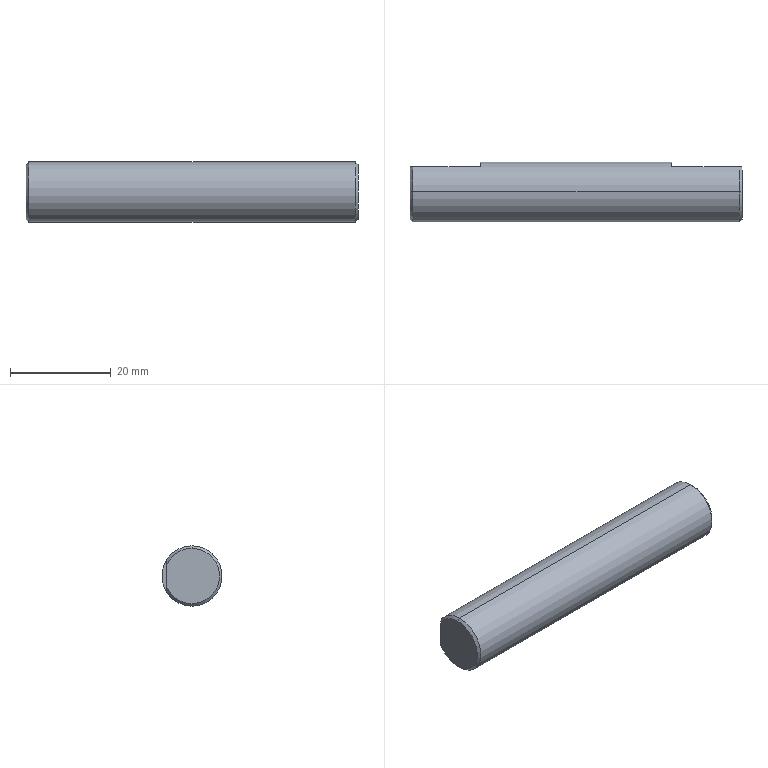Part | SolidWorks | features BaseBody 1 | 1 solid | 14 faces | box 66 x 12 x 12 mm | volume 7331 mm3 | cone 6 | plane 6 | cylinder 2 | commonest cylinder face diameters 12 x2
STEP:
#1=CARTESIAN_POINT('',(65.5,5.,-3.317));
#2=VERTEX_POINT('',#1);
#3=CARTESIAN_POINT('',(65.5,0.,-6.));
#4=VERTEX_POINT('',#3);
#5=CARTESIAN_POINT('',(65.5,0.,0.));
#6=DIRECTION('',(-1.,0.,0.));
#7=DIRECTION('',(0.,0.,1.));
#8=AXIS2_PLACEMENT_3D('',#5,#6,#7);
#9=CIRCLE('',#8,6.);
#10=EDGE_CURVE('',#2,#4,#9,.T.);
#11=ORIENTED_EDGE('',*,*,#10,.T.);
#12=CARTESIAN_POINT('',(0.5,0.,-6.));
#13=VERTEX_POINT('',#12);
#14=CARTESIAN_POINT('',(0.,0.,-6.));
#15=DIRECTION('',(-1.,0.,0.));
#16=VECTOR('',#15,1000.);
#17=LINE('',#14,#16);
#18=EDGE_CURVE('',#4,#13,#17,.T.);
#19=ORIENTED_EDGE('',*,*,#18,.T.);
#20=CARTESIAN_POINT('',(0.5,5.,-3.317));
#21=VERTEX_POINT('',#20);
#22=CARTESIAN_POINT('',(0.5,0.,0.));
#23=DIRECTION('',(1.,0.,0.));
#24=DIRECTION('',(0.,0.,1.));
#25=AXIS2_PLACEMENT_3D('',#22,#23,#24);
#26=CIRCLE('',#25,6.);
#27=EDGE_CURVE('',#13,#21,#26,.T.);
#28=ORIENTED_EDGE('',*,*,#27,.T.);
#29=CARTESIAN_POINT('',(14.,5.,-3.317));
#30=VERTEX_POINT('',#29);
#31=CARTESIAN_POINT('',(0.,5.,-3.317));
#32=DIRECTION('',(1.,0.,0.));
#33=VECTOR('',#32,1000.);
#34=LINE('',#31,#33);
#35=EDGE_CURVE('',#21,#30,#34,.T.);
#36=ORIENTED_EDGE('',*,*,#35,.T.);
#37=CARTESIAN_POINT('',(14.,5.,3.317));
#38=VERTEX_POINT('',#37);
#39=CARTESIAN_POINT('',(14.,0.,0.));
#40=DIRECTION('',(1.,0.,0.));
#41=DIRECTION('',(0.,0.,1.));
#42=AXIS2_PLACEMENT_3D('',#39,#40,#41);
#43=CIRCLE('',#42,6.);
#44=EDGE_CURVE('',#30,#38,#43,.T.);
#45=ORIENTED_EDGE('',*,*,#44,.T.);
#46=CARTESIAN_POINT('',(0.5,5.,3.317));
#47=VERTEX_POINT('',#46);
#48=CARTESIAN_POINT('',(0.,5.,3.317));
#49=DIRECTION('',(-1.,0.,0.));
#50=VECTOR('',#49,1000.);
#51=LINE('',#48,#50);
#52=EDGE_CURVE('',#38,#47,#51,.T.);
#53=ORIENTED_EDGE('',*,*,#52,.T.);
#54=CARTESIAN_POINT('',(0.5,0.,6.));
#55=VERTEX_POINT('',#54);
#56=CARTESIAN_POINT('',(0.5,0.,0.));
#57=DIRECTION('',(1.,0.,0.));
#58=DIRECTION('',(0.,0.,1.));
#59=AXIS2_PLACEMENT_3D('',#56,#57,#58);
#60=CIRCLE('',#59,6.);
#61=EDGE_CURVE('',#47,#55,#60,.T.);
#62=ORIENTED_EDGE('',*,*,#61,.T.);
#63=CARTESIAN_POINT('',(65.5,0.,6.));
#64=VERTEX_POINT('',#63);
#65=CARTESIAN_POINT('',(0.,0.,6.));
#66=DIRECTION('',(-1.,0.,0.));
#67=VECTOR('',#66,1000.);
#68=LINE('',#65,#67);
#69=EDGE_CURVE('',#64,#55,#68,.T.);
#70=ORIENTED_EDGE('',*,*,#69,.F.);
#71=CARTESIAN_POINT('',(65.5,5.,3.317));
#72=VERTEX_POINT('',#71);
#73=CARTESIAN_POINT('',(65.5,0.,0.));
#74=DIRECTION('',(-1.,0.,0.));
#75=DIRECTION('',(0.,0.,1.));
#76=AXIS2_PLACEMENT_3D('',#73,#74,#75);
#77=CIRCLE('',#76,6.);
#78=EDGE_CURVE('',#64,#72,#77,.T.);
#79=ORIENTED_EDGE('',*,*,#78,.T.);
#80=CARTESIAN_POINT('',(52.,5.,3.317));
#81=VERTEX_POINT('',#80);
#82=CARTESIAN_POINT('',(0.,5.,3.317));
#83=DIRECTION('',(-1.,0.,0.));
#84=VECTOR('',#83,1000.);
#85=LINE('',#82,#84);
#86=EDGE_CURVE('',#72,#81,#85,.T.);
#87=ORIENTED_EDGE('',*,*,#86,.T.);
#88=CARTESIAN_POINT('',(52.,5.,-3.317));
#89=VERTEX_POINT('',#88);
#90=CARTESIAN_POINT('',(52.,0.,0.));
#91=DIRECTION('',(-1.,0.,0.));
#92=DIRECTION('',(0.,0.,1.));
#93=AXIS2_PLACEMENT_3D('',#90,#91,#92);
#94=CIRCLE('',#93,6.);
#95=EDGE_CURVE('',#81,#89,#94,.T.);
#96=ORIENTED_EDGE('',*,*,#95,.T.);
#97=CARTESIAN_POINT('',(0.,5.,-3.317));
#98=DIRECTION('',(1.,0.,0.));
#99=VECTOR('',#98,1000.);
#100=LINE('',#97,#99);
#101=EDGE_CURVE('',#89,#2,#100,.T.);
#102=ORIENTED_EDGE('',*,*,#101,.T.);
#103=EDGE_LOOP('',(#11,#19,#28,#36,#45,#53,#62,#70,#79,#87,#96,#102));
#104=FACE_OUTER_BOUND('',#103,.T.);
#105=CARTESIAN_POINT('',(0.,0.,0.));
#106=DIRECTION('',(-1.,0.,0.));
#107=DIRECTION('',(0.,0.,1.));
#108=AXIS2_PLACEMENT_3D('',#105,#106,#107);
#109=CYLINDRICAL_SURFACE('',#108,6.);
#110=ADVANCED_FACE('',(#104),#109,.T.);
#111=CARTESIAN_POINT('',(0.,5.,2.291));
#112=VERTEX_POINT('',#111);
#113=CARTESIAN_POINT('',(0.,0.,5.5));
#114=VERTEX_POINT('',#113);
#115=CARTESIAN_POINT('',(0.,0.,0.));
#116=DIRECTION('',(1.,0.,0.));
#117=DIRECTION('',(0.,0.,-1.));
#118=AXIS2_PLACEMENT_3D('',#115,#116,#117);
#119=CIRCLE('',#118,5.5);
#120=EDGE_CURVE('',#112,#114,#119,.T.);
#121=ORIENTED_EDGE('',*,*,#120,.T.);
#122=CARTESIAN_POINT('',(0.5,0.,6.));
#123=DIRECTION('',(0.7071,0.,0.7071));
#124=VECTOR('',#123,1000.);
#125=LINE('',#122,#124);
#126=EDGE_CURVE('',#114,#55,#125,.T.);
#127=ORIENTED_EDGE('',*,*,#126,.T.);
#128=ORIENTED_EDGE('',*,*,#61,.F.);
#129=CARTESIAN_POINT('',(0.5,5.,3.317));
#130=CARTESIAN_POINT('',(0.3158,5.,2.983));
#131=CARTESIAN_POINT('',(0.1465,5.,2.643));
#132=CARTESIAN_POINT('',(0.,5.,2.291));
#133=B_SPLINE_CURVE_WITH_KNOTS('',3,(#129,#130,#131,#132),.UNSPECIFIED.,.F.,.F.,(4,4),(0.,0.001141),.UNSPECIFIED.);
#134=EDGE_CURVE('',#47,#112,#133,.T.);
#135=ORIENTED_EDGE('',*,*,#134,.T.);
#136=EDGE_LOOP('',(#121,#127,#128,#135));
#137=FACE_OUTER_BOUND('',#136,.T.);
#138=CARTESIAN_POINT('',(0.5,0.,0.));
#139=DIRECTION('',(1.,0.,0.));
#140=DIRECTION('',(0.,0.,-1.));
#141=AXIS2_PLACEMENT_3D('',#138,#139,#140);
#142=CONICAL_SURFACE('',#141,6.,0.7854);
#143=ADVANCED_FACE('',(#137),#142,.T.);
#144=ORIENTED_EDGE('',*,*,#126,.F.);
#145=CARTESIAN_POINT('',(0.,0.,-5.5));
#146=VERTEX_POINT('',#145);
#147=CARTESIAN_POINT('',(0.,0.,0.));
#148=DIRECTION('',(1.,0.,0.));
#149=DIRECTION('',(0.,0.,-1.));
#150=AXIS2_PLACEMENT_3D('',#147,#148,#149);
#151=CIRCLE('',#150,5.5);
#152=EDGE_CURVE('',#114,#146,#151,.T.);
#153=ORIENTED_EDGE('',*,*,#152,.T.);
#154=CARTESIAN_POINT('',(0.5,0.,-6.));
#155=DIRECTION('',(0.7071,0.,-0.7071));
#156=VECTOR('',#155,1000.);
#157=LINE('',#154,#156);
#158=EDGE_CURVE('',#146,#13,#157,.T.);
#159=ORIENTED_EDGE('',*,*,#158,.T.);
#160=CARTESIAN_POINT('',(0.5,0.,0.));
#161=DIRECTION('',(1.,0.,0.));
#162=DIRECTION('',(0.,0.,1.));
#163=AXIS2_PLACEMENT_3D('',#160,#161,#162);
#164=CIRCLE('',#163,6.);
#165=EDGE_CURVE('',#55,#13,#164,.T.);
#166=ORIENTED_EDGE('',*,*,#165,.F.);
#167=EDGE_LOOP('',(#144,#153,#159,#166));
#168=FACE_OUTER_BOUND('',#167,.T.);
#169=CARTESIAN_POINT('',(0.5,0.,0.));
#170=DIRECTION('',(1.,0.,0.));
#171=DIRECTION('',(0.,0.,-1.));
#172=AXIS2_PLACEMENT_3D('',#169,#170,#171);
#173=CONICAL_SURFACE('',#172,6.,0.7854);
#174=ADVANCED_FACE('',(#168),#173,.T.);
#175=CARTESIAN_POINT('',(66.,5.,-2.291));
#176=VERTEX_POINT('',#175);
#177=CARTESIAN_POINT('',(66.,0.,-5.5));
#178=VERTEX_POINT('',#177);
#179=CARTESIAN_POINT('',(66.,0.,0.));
#180=DIRECTION('',(-1.,0.,0.));
#181=DIRECTION('',(0.,0.,1.));
#182=AXIS2_PLACEMENT_3D('',#179,#180,#181);
#183=CIRCLE('',#182,5.5);
#184=EDGE_CURVE('',#176,#178,#183,.T.);
#185=ORIENTED_EDGE('',*,*,#184,.T.);
#186=CARTESIAN_POINT('',(65.5,0.,-6.));
#187=DIRECTION('',(-0.7071,0.,-0.7071));
#188=VECTOR('',#187,1000.);
#189=LINE('',#186,#188);
#190=EDGE_CURVE('',#178,#4,#189,.T.);
#191=ORIENTED_EDGE('',*,*,#190,.T.);
#192=ORIENTED_EDGE('',*,*,#10,.F.);
#193=CARTESIAN_POINT('',(65.5,5.,-3.317));
#194=CARTESIAN_POINT('',(65.684,5.,-2.983));
#195=CARTESIAN_POINT('',(65.854,5.,-2.643));
#196=CARTESIAN_POINT('',(66.,5.,-2.291));
#197=B_SPLINE_CURVE_WITH_KNOTS('',3,(#193,#194,#195,#196),.UNSPECIFIED.,.F.,.F.,(4,4),(0.,0.001141),.UNSPECIFIED.);
#198=EDGE_CURVE('',#2,#176,#197,.T.);
#199=ORIENTED_EDGE('',*,*,#198,.T.);
#200=EDGE_LOOP('',(#185,#191,#192,#199));
#201=FACE_OUTER_BOUND('',#200,.T.);
#202=CARTESIAN_POINT('',(65.5,0.,0.));
#203=DIRECTION('',(-1.,0.,0.));
#204=DIRECTION('',(0.,0.,1.));
#205=AXIS2_PLACEMENT_3D('',#202,#203,#204);
#206=CONICAL_SURFACE('',#205,6.,0.7854);
#207=ADVANCED_FACE('',(#201),#206,.T.);
#208=ORIENTED_EDGE('',*,*,#190,.F.);
#209=CARTESIAN_POINT('',(66.,0.,5.5));
#210=VERTEX_POINT('',#209);
#211=CARTESIAN_POINT('',(66.,0.,0.));
#212=DIRECTION('',(-1.,0.,0.));
#213=DIRECTION('',(0.,0.,1.));
#214=AXIS2_PLACEMENT_3D('',#211,#212,#213);
#215=CIRCLE('',#214,5.5);
#216=EDGE_CURVE('',#178,#210,#215,.T.);
#217=ORIENTED_EDGE('',*,*,#216,.T.);
#218=CARTESIAN_POINT('',(65.5,0.,6.));
#219=DIRECTION('',(-0.7071,0.,0.7071));
#220=VECTOR('',#219,1000.);
#221=LINE('',#218,#220);
#222=EDGE_CURVE('',#210,#64,#221,.T.);
#223=ORIENTED_EDGE('',*,*,#222,.T.);
#224=CARTESIAN_POINT('',(65.5,0.,0.));
#225=DIRECTION('',(-1.,0.,0.));
#226=DIRECTION('',(0.,0.,1.));
#227=AXIS2_PLACEMENT_3D('',#224,#225,#226);
#228=CIRCLE('',#227,6.);
#229=EDGE_CURVE('',#4,#64,#228,.T.);
#230=ORIENTED_EDGE('',*,*,#229,.F.);
#231=EDGE_LOOP('',(#208,#217,#223,#230));
#232=FACE_OUTER_BOUND('',#231,.T.);
#233=CARTESIAN_POINT('',(65.5,0.,0.));
#234=DIRECTION('',(-1.,0.,0.));
#235=DIRECTION('',(0.,0.,1.));
#236=AXIS2_PLACEMENT_3D('',#233,#234,#235);
#237=CONICAL_SURFACE('',#236,6.,0.7854);
#238=ADVANCED_FACE('',(#232),#237,.T.);
#239=ORIENTED_EDGE('',*,*,#18,.F.);
#240=ORIENTED_EDGE('',*,*,#229,.T.);
#241=ORIENTED_EDGE('',*,*,#69,.T.);
#242=ORIENTED_EDGE('',*,*,#165,.T.);
#243=EDGE_LOOP('',(#239,#240,#241,#242));
#244=FACE_OUTER_BOUND('',#243,.T.);
#245=CARTESIAN_POINT('',(0.,0.,0.));
#246=DIRECTION('',(-1.,0.,0.));
#247=DIRECTION('',(0.,0.,1.));
#248=AXIS2_PLACEMENT_3D('',#245,#246,#247);
#249=CYLINDRICAL_SURFACE('',#248,6.);
#250=ADVANCED_FACE('',(#244),#249,.T.);
#251=ORIENTED_EDGE('',*,*,#158,.F.);
#252=CARTESIAN_POINT('',(0.,5.,-2.291));
#253=VERTEX_POINT('',#252);
#254=CARTESIAN_POINT('',(0.,0.,0.));
#255=DIRECTION('',(1.,0.,0.));
#256=DIRECTION('',(0.,0.,-1.));
#257=AXIS2_PLACEMENT_3D('',#254,#255,#256);
#258=CIRCLE('',#257,5.5);
#259=EDGE_CURVE('',#146,#253,#258,.T.);
#260=ORIENTED_EDGE('',*,*,#259,.T.);
#261=CARTESIAN_POINT('',(0.,5.,-2.291));
#262=CARTESIAN_POINT('',(0.1465,5.,-2.643));
#263=CARTESIAN_POINT('',(0.3158,5.,-2.983));
#264=CARTESIAN_POINT('',(0.5,5.,-3.317));
#265=B_SPLINE_CURVE_WITH_KNOTS('',3,(#261,#262,#263,#264),.UNSPECIFIED.,.F.,.F.,(4,4),(0.,0.001141),.UNSPECIFIED.);
#266=EDGE_CURVE('',#253,#21,#265,.T.);
#267=ORIENTED_EDGE('',*,*,#266,.T.);
#268=ORIENTED_EDGE('',*,*,#27,.F.);
#269=EDGE_LOOP('',(#251,#260,#267,#268));
#270=FACE_OUTER_BOUND('',#269,.T.);
#271=CARTESIAN_POINT('',(0.5,0.,0.));
#272=DIRECTION('',(1.,0.,0.));
#273=DIRECTION('',(0.,0.,-1.));
#274=AXIS2_PLACEMENT_3D('',#271,#272,#273);
#275=CONICAL_SURFACE('',#274,6.,0.7854);
#276=ADVANCED_FACE('',(#270),#275,.T.);
#277=ORIENTED_EDGE('',*,*,#222,.F.);
#278=CARTESIAN_POINT('',(66.,5.,2.291));
#279=VERTEX_POINT('',#278);
#280=CARTESIAN_POINT('',(66.,0.,0.));
#281=DIRECTION('',(-1.,0.,0.));
#282=DIRECTION('',(0.,0.,1.));
#283=AXIS2_PLACEMENT_3D('',#280,#281,#282);
#284=CIRCLE('',#283,5.5);
#285=EDGE_CURVE('',#210,#279,#284,.T.);
#286=ORIENTED_EDGE('',*,*,#285,.T.);
#287=CARTESIAN_POINT('',(66.,5.,2.291));
#288=CARTESIAN_POINT('',(65.854,5.,2.643));
#289=CARTESIAN_POINT('',(65.684,5.,2.983));
#290=CARTESIAN_POINT('',(65.5,5.,3.317));
#291=B_SPLINE_CURVE_WITH_KNOTS('',3,(#287,#288,#289,#290),.UNSPECIFIED.,.F.,.F.,(4,4),(0.,0.001141),.UNSPECIFIED.);
#292=EDGE_CURVE('',#279,#72,#291,.T.);
#293=ORIENTED_EDGE('',*,*,#292,.T.);
#294=ORIENTED_EDGE('',*,*,#78,.F.);
#295=EDGE_LOOP('',(#277,#286,#293,#294));
#296=FACE_OUTER_BOUND('',#295,.T.);
#297=CARTESIAN_POINT('',(65.5,0.,0.));
#298=DIRECTION('',(-1.,0.,0.));
#299=DIRECTION('',(0.,0.,1.));
#300=AXIS2_PLACEMENT_3D('',#297,#298,#299);
#301=CONICAL_SURFACE('',#300,6.,0.7854);
#302=ADVANCED_FACE('',(#296),#301,.T.);
#303=CARTESIAN_POINT('',(0.,5.,0.));
#304=DIRECTION('',(0.,0.,1.));
#305=VECTOR('',#304,1000.);
#306=LINE('',#303,#305);
#307=EDGE_CURVE('',#253,#112,#306,.T.);
#308=ORIENTED_EDGE('',*,*,#307,.F.);
#309=ORIENTED_EDGE('',*,*,#259,.F.);
#310=ORIENTED_EDGE('',*,*,#152,.F.);
#311=ORIENTED_EDGE('',*,*,#120,.F.);
#312=EDGE_LOOP('',(#308,#309,#310,#311));
#313=FACE_OUTER_BOUND('',#312,.T.);
#314=CARTESIAN_POINT('',(0.,0.,0.));
#315=DIRECTION('',(1.,0.,0.));
#316=DIRECTION('',(0.,0.,-1.));
#317=AXIS2_PLACEMENT_3D('',#314,#315,#316);
#318=PLANE('',#317);
#319=ADVANCED_FACE('',(#313),#318,.F.);
#320=ORIENTED_EDGE('',*,*,#292,.F.);
#321=CARTESIAN_POINT('',(66.,5.,-5.));
#322=DIRECTION('',(0.,0.,1.));
#323=VECTOR('',#322,1000.);
#324=LINE('',#321,#323);
#325=EDGE_CURVE('',#176,#279,#324,.T.);
#326=ORIENTED_EDGE('',*,*,#325,.F.);
#327=ORIENTED_EDGE('',*,*,#198,.F.);
#328=ORIENTED_EDGE('',*,*,#101,.F.);
#329=CARTESIAN_POINT('',(52.,5.,-5.));
#330=DIRECTION('',(0.,0.,-1.));
#331=VECTOR('',#330,1000.);
#332=LINE('',#329,#331);
#333=EDGE_CURVE('',#81,#89,#332,.T.);
#334=ORIENTED_EDGE('',*,*,#333,.F.);
#335=ORIENTED_EDGE('',*,*,#86,.F.);
#336=EDGE_LOOP('',(#320,#326,#327,#328,#334,#335));
#337=FACE_OUTER_BOUND('',#336,.T.);
#338=CARTESIAN_POINT('',(68.507,5.,-5.));
#339=DIRECTION('',(0.,-1.,0.));
#340=DIRECTION('',(1.,0.,0.));
#341=AXIS2_PLACEMENT_3D('',#338,#339,#340);
#342=PLANE('',#341);
#343=ADVANCED_FACE('',(#337),#342,.F.);
#344=ORIENTED_EDGE('',*,*,#95,.F.);
#345=ORIENTED_EDGE('',*,*,#333,.T.);
#346=EDGE_LOOP('',(#344,#345));
#347=FACE_OUTER_BOUND('',#346,.T.);
#348=CARTESIAN_POINT('',(52.,7.754,-5.));
#349=DIRECTION('',(-1.,0.,0.));
#350=DIRECTION('',(0.,0.,1.));
#351=AXIS2_PLACEMENT_3D('',#348,#349,#350);
#352=PLANE('',#351);
#353=ADVANCED_FACE('',(#347),#352,.F.);
#354=ORIENTED_EDGE('',*,*,#134,.F.);
#355=ORIENTED_EDGE('',*,*,#52,.F.);
#356=CARTESIAN_POINT('',(14.,5.,-5.));
#357=DIRECTION('',(0.,0.,1.));
#358=VECTOR('',#357,1000.);
#359=LINE('',#356,#358);
#360=EDGE_CURVE('',#30,#38,#359,.T.);
#361=ORIENTED_EDGE('',*,*,#360,.F.);
#362=ORIENTED_EDGE('',*,*,#35,.F.);
#363=ORIENTED_EDGE('',*,*,#266,.F.);
#364=ORIENTED_EDGE('',*,*,#307,.T.);
#365=EDGE_LOOP('',(#354,#355,#361,#362,#363,#364));
#366=FACE_OUTER_BOUND('',#365,.T.);
#367=CARTESIAN_POINT('',(-2.419,5.,-5.));
#368=DIRECTION('',(0.,-1.,0.));
#369=DIRECTION('',(0.,0.,-1.));
#370=AXIS2_PLACEMENT_3D('',#367,#368,#369);
#371=PLANE('',#370);
#372=ADVANCED_FACE('',(#366),#371,.F.);
#373=ORIENTED_EDGE('',*,*,#44,.F.);
#374=ORIENTED_EDGE('',*,*,#360,.T.);
#375=EDGE_LOOP('',(#373,#374));
#376=FACE_OUTER_BOUND('',#375,.T.);
#377=CARTESIAN_POINT('',(14.,10.401,-5.));
#378=DIRECTION('',(1.,0.,0.));
#379=DIRECTION('',(0.,1.,0.));
#380=AXIS2_PLACEMENT_3D('',#377,#378,#379);
#381=PLANE('',#380);
#382=ADVANCED_FACE('',(#376),#381,.F.);
#383=ORIENTED_EDGE('',*,*,#325,.T.);
#384=ORIENTED_EDGE('',*,*,#285,.F.);
#385=ORIENTED_EDGE('',*,*,#216,.F.);
#386=ORIENTED_EDGE('',*,*,#184,.F.);
#387=EDGE_LOOP('',(#383,#384,#385,#386));
#388=FACE_OUTER_BOUND('',#387,.T.);
#389=CARTESIAN_POINT('',(66.,6.,0.));
#390=DIRECTION('',(-1.,0.,0.));
#391=DIRECTION('',(0.,0.,1.));
#392=AXIS2_PLACEMENT_3D('',#389,#390,#391);
#393=PLANE('',#392);
#394=ADVANCED_FACE('',(#388),#393,.F.);
#395=CLOSED_SHELL('',(#110,#143,#174,#207,#238,#250,#276,#302,#319,#343,#353,#372,#382,#394));
#396=MANIFOLD_SOLID_BREP('',#395);
#397=CARTESIAN_POINT('',(0.,0.,0.));
#398=DIRECTION('',(0.,0.,1.));
#399=DIRECTION('',(1.,0.,0.));
#400=AXIS2_PLACEMENT_3D('',#397,#398,#399);
#401=(LENGTH_UNIT()NAMED_UNIT(*)SI_UNIT(.MILLI.,.METRE.));
#402=UNCERTAINTY_MEASURE_WITH_UNIT(LENGTH_MEASURE(0.00001),#401,'','');
#403=(NAMED_UNIT(*)PLANE_ANGLE_UNIT()SI_UNIT($,.RADIAN.));
#404=(NAMED_UNIT(*)SI_UNIT($,.STERADIAN.)SOLID_ANGLE_UNIT());
#405=(GEOMETRIC_REPRESENTATION_CONTEXT(3)GLOBAL_UNCERTAINTY_ASSIGNED_CONTEXT((#402))GLOBAL_UNIT_ASSIGNED_CONTEXT((#401,#403,#404))REPRESENTATION_CONTEXT('',''));
#406=ADVANCED_BREP_SHAPE_REPRESENTATION('',(#396,#400),#405);